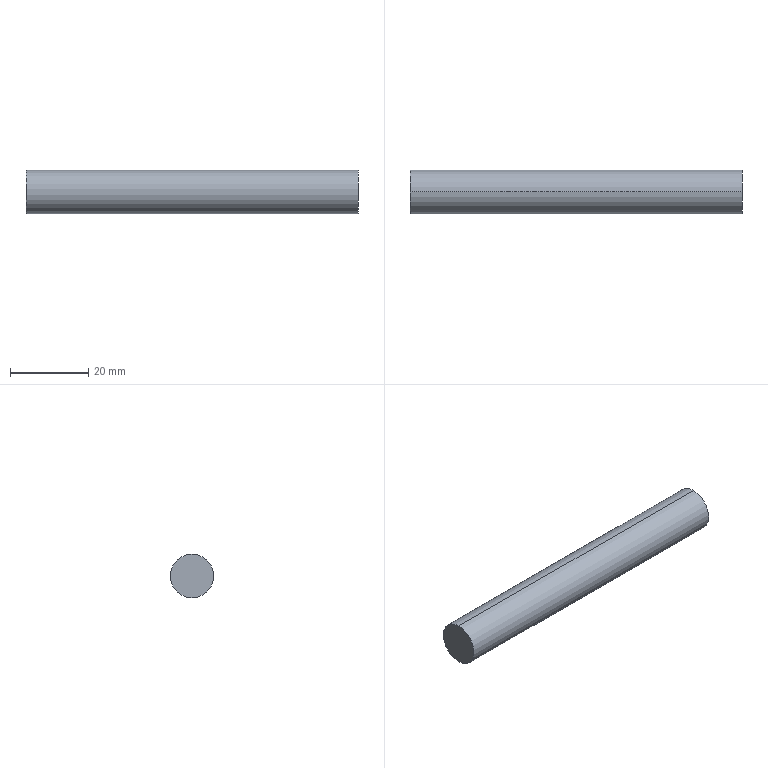Part | STEP file | 4-20.sldasm-Part-385 | 1 solid | 4 faces | box 85 x 11.11 x 11.11 mm | volume 8240 mm3 | cylinder 2 | plane 2 | commonest cylinder face diameters 11.11 x2
STEP:
#1=CARTESIAN_POINT('',(40.,60.,179.555));
#2=VERTEX_POINT('',#1);
#3=CARTESIAN_POINT('',(40.,60.,168.445));
#4=VERTEX_POINT('',#3);
#5=CARTESIAN_POINT('',(40.,60.,174.));
#6=DIRECTION('',(1.,0.,0.));
#7=DIRECTION('',(0.,0.,1.));
#8=AXIS2_PLACEMENT_3D('',#5,#6,#7);
#9=CIRCLE('',#8,5.555);
#10=EDGE_CURVE('',#2,#4,#9,.T.);
#11=ORIENTED_EDGE('',*,*,#10,.T.);
#12=CARTESIAN_POINT('',(125.,60.,168.445));
#13=VERTEX_POINT('',#12);
#14=CARTESIAN_POINT('',(50.,60.,168.445));
#15=DIRECTION('',(1.,0.,0.));
#16=VECTOR('',#15,1000.);
#17=LINE('',#14,#16);
#18=EDGE_CURVE('',#4,#13,#17,.T.);
#19=ORIENTED_EDGE('',*,*,#18,.T.);
#20=CARTESIAN_POINT('',(125.,60.,179.555));
#21=VERTEX_POINT('',#20);
#22=CARTESIAN_POINT('',(125.,60.,174.));
#23=DIRECTION('',(-1.,0.,0.));
#24=DIRECTION('',(0.,0.,-1.));
#25=AXIS2_PLACEMENT_3D('',#22,#23,#24);
#26=CIRCLE('',#25,5.555);
#27=EDGE_CURVE('',#13,#21,#26,.T.);
#28=ORIENTED_EDGE('',*,*,#27,.T.);
#29=CARTESIAN_POINT('',(50.,60.,179.555));
#30=DIRECTION('',(1.,0.,0.));
#31=VECTOR('',#30,1000.);
#32=LINE('',#29,#31);
#33=EDGE_CURVE('',#2,#21,#32,.T.);
#34=ORIENTED_EDGE('',*,*,#33,.F.);
#35=EDGE_LOOP('',(#11,#19,#28,#34));
#36=FACE_OUTER_BOUND('',#35,.T.);
#37=CARTESIAN_POINT('',(50.,60.,174.));
#38=DIRECTION('',(1.,0.,0.));
#39=DIRECTION('',(0.,0.,1.));
#40=AXIS2_PLACEMENT_3D('',#37,#38,#39);
#41=CYLINDRICAL_SURFACE('',#40,5.555);
#42=ADVANCED_FACE('',(#36),#41,.T.);
#43=ORIENTED_EDGE('',*,*,#18,.F.);
#44=CARTESIAN_POINT('',(40.,60.,174.));
#45=DIRECTION('',(1.,0.,0.));
#46=DIRECTION('',(0.,0.,1.));
#47=AXIS2_PLACEMENT_3D('',#44,#45,#46);
#48=CIRCLE('',#47,5.555);
#49=EDGE_CURVE('',#4,#2,#48,.T.);
#50=ORIENTED_EDGE('',*,*,#49,.T.);
#51=ORIENTED_EDGE('',*,*,#33,.T.);
#52=CARTESIAN_POINT('',(125.,60.,174.));
#53=DIRECTION('',(-1.,0.,0.));
#54=DIRECTION('',(0.,0.,-1.));
#55=AXIS2_PLACEMENT_3D('',#52,#53,#54);
#56=CIRCLE('',#55,5.555);
#57=EDGE_CURVE('',#21,#13,#56,.T.);
#58=ORIENTED_EDGE('',*,*,#57,.T.);
#59=EDGE_LOOP('',(#43,#50,#51,#58));
#60=FACE_OUTER_BOUND('',#59,.T.);
#61=CARTESIAN_POINT('',(50.,60.,174.));
#62=DIRECTION('',(1.,0.,0.));
#63=DIRECTION('',(0.,0.,1.));
#64=AXIS2_PLACEMENT_3D('',#61,#62,#63);
#65=CYLINDRICAL_SURFACE('',#64,5.555);
#66=ADVANCED_FACE('',(#60),#65,.T.);
#67=ORIENTED_EDGE('',*,*,#10,.F.);
#68=ORIENTED_EDGE('',*,*,#49,.F.);
#69=EDGE_LOOP('',(#67,#68));
#70=FACE_OUTER_BOUND('',#69,.T.);
#71=CARTESIAN_POINT('',(40.,60.,174.));
#72=DIRECTION('',(-1.,0.,0.));
#73=DIRECTION('',(0.,0.,-1.));
#74=AXIS2_PLACEMENT_3D('',#71,#72,#73);
#75=PLANE('',#74);
#76=ADVANCED_FACE('',(#70),#75,.T.);
#77=ORIENTED_EDGE('',*,*,#57,.F.);
#78=ORIENTED_EDGE('',*,*,#27,.F.);
#79=EDGE_LOOP('',(#77,#78));
#80=FACE_OUTER_BOUND('',#79,.T.);
#81=CARTESIAN_POINT('',(125.,-310.,374.));
#82=DIRECTION('',(1.,0.,0.));
#83=DIRECTION('',(0.,0.,-1.));
#84=AXIS2_PLACEMENT_3D('',#81,#82,#83);
#85=PLANE('',#84);
#86=ADVANCED_FACE('',(#80),#85,.T.);
#87=CLOSED_SHELL('',(#42,#66,#76,#86));
#88=MANIFOLD_SOLID_BREP('',#87);
#89=CARTESIAN_POINT('',(0.,0.,0.));
#90=DIRECTION('',(0.,0.,1.));
#91=DIRECTION('',(1.,0.,0.));
#92=AXIS2_PLACEMENT_3D('',#89,#90,#91);
#93=(LENGTH_UNIT()NAMED_UNIT(*)SI_UNIT(.MILLI.,.METRE.));
#94=UNCERTAINTY_MEASURE_WITH_UNIT(LENGTH_MEASURE(0.00001),#93,'','');
#95=(NAMED_UNIT(*)PLANE_ANGLE_UNIT()SI_UNIT($,.RADIAN.));
#96=(NAMED_UNIT(*)SI_UNIT($,.STERADIAN.)SOLID_ANGLE_UNIT());
#97=(GEOMETRIC_REPRESENTATION_CONTEXT(3)GLOBAL_UNCERTAINTY_ASSIGNED_CONTEXT((#94))GLOBAL_UNIT_ASSIGNED_CONTEXT((#93,#95,#96))REPRESENTATION_CONTEXT('',''));
#98=ADVANCED_BREP_SHAPE_REPRESENTATION('',(#88,#92),#97);